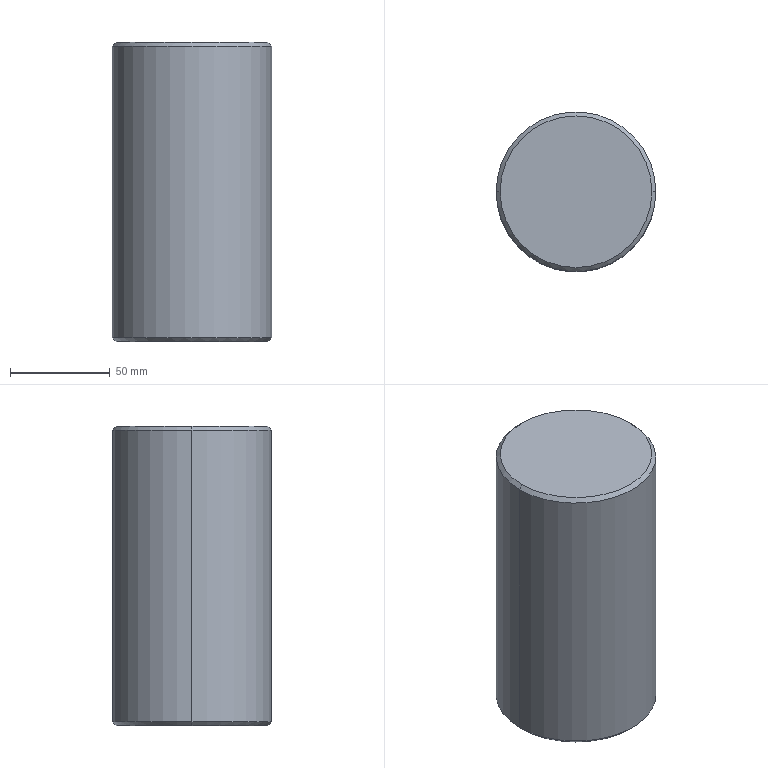Part | Creo | 1 solid | 15 faces | box 80 x 80 x 150 mm | volume 750871 mm3 | cylinder 6 | cone 6 | plane 3 | commonest cylinder face diameters 10.199 x2 10.2 x2 80 x2
STEP:
#1=CARTESIAN_POINT('',(-40.,-165.,-268.5));
#2=VERTEX_POINT('',#1);
#3=CARTESIAN_POINT('',(40.,-165.,-268.5));
#4=VERTEX_POINT('',#3);
#5=CARTESIAN_POINT('',(0.,-165.,-268.5));
#6=DIRECTION('',(0.,0.,-1.));
#7=DIRECTION('',(-1.,0.,0.));
#8=AXIS2_PLACEMENT_3D('',#5,#6,#7);
#9=CIRCLE('',#8,40.);
#10=EDGE_CURVE('',#2,#4,#9,.T.);
#11=ORIENTED_EDGE('',*,*,#10,.T.);
#12=CARTESIAN_POINT('',(40.,-165.,-122.5));
#13=VERTEX_POINT('',#12);
#14=CARTESIAN_POINT('',(40.,-165.,-122.5));
#15=DIRECTION('',(0.,0.,-1.));
#16=VECTOR('',#15,146.);
#17=LINE('',#14,#16);
#18=EDGE_CURVE('',#13,#4,#17,.T.);
#19=ORIENTED_EDGE('',*,*,#18,.F.);
#20=CARTESIAN_POINT('',(-40.,-165.,-122.5));
#21=VERTEX_POINT('',#20);
#22=CARTESIAN_POINT('',(0.,-165.,-122.5));
#23=DIRECTION('',(0.,0.,1.));
#24=DIRECTION('',(1.,0.,0.));
#25=AXIS2_PLACEMENT_3D('',#22,#23,#24);
#26=CIRCLE('',#25,40.);
#27=EDGE_CURVE('',#13,#21,#26,.T.);
#28=ORIENTED_EDGE('',*,*,#27,.T.);
#29=CARTESIAN_POINT('',(-40.,-165.,-122.5));
#30=DIRECTION('',(0.,0.,-1.));
#31=VECTOR('',#30,146.);
#32=LINE('',#29,#31);
#33=EDGE_CURVE('',#21,#2,#32,.T.);
#34=ORIENTED_EDGE('',*,*,#33,.T.);
#35=EDGE_LOOP('',(#11,#19,#28,#34));
#36=FACE_OUTER_BOUND('',#35,.F.);
#37=CARTESIAN_POINT('',(0.,-165.,-120.5));
#38=DIRECTION('',(0.,0.,-1.));
#39=DIRECTION('',(-1.,0.,0.));
#40=AXIS2_PLACEMENT_3D('',#37,#38,#39);
#41=CYLINDRICAL_SURFACE('',#40,40.);
#42=ADVANCED_FACE('',(#36),#41,.T.);
#43=CARTESIAN_POINT('',(-38.,-165.,-270.5));
#44=VERTEX_POINT('',#43);
#45=CARTESIAN_POINT('',(38.,-165.,-270.5));
#46=VERTEX_POINT('',#45);
#47=CARTESIAN_POINT('',(0.,-165.,-270.5));
#48=DIRECTION('',(0.,0.,-1.));
#49=DIRECTION('',(-1.,0.,0.));
#50=AXIS2_PLACEMENT_3D('',#47,#48,#49);
#51=CIRCLE('',#50,38.);
#52=EDGE_CURVE('',#44,#46,#51,.T.);
#53=ORIENTED_EDGE('',*,*,#52,.T.);
#54=CARTESIAN_POINT('',(38.,-165.,-270.5));
#55=DIRECTION('',(0.7071,0.,0.7071));
#56=VECTOR('',#55,2.828);
#57=LINE('',#54,#56);
#58=EDGE_CURVE('',#46,#4,#57,.T.);
#59=ORIENTED_EDGE('',*,*,#58,.T.);
#60=ORIENTED_EDGE('',*,*,#10,.F.);
#61=CARTESIAN_POINT('',(-38.,-165.,-270.5));
#62=DIRECTION('',(-0.7071,0.,0.7071));
#63=VECTOR('',#62,2.828);
#64=LINE('',#61,#63);
#65=EDGE_CURVE('',#44,#2,#64,.T.);
#66=ORIENTED_EDGE('',*,*,#65,.F.);
#67=EDGE_LOOP('',(#53,#59,#60,#66));
#68=FACE_OUTER_BOUND('',#67,.F.);
#69=CARTESIAN_POINT('',(0.,-165.,-269.5));
#70=DIRECTION('',(0.,0.,1.));
#71=DIRECTION('',(1.,0.,0.));
#72=AXIS2_PLACEMENT_3D('',#69,#70,#71);
#73=CONICAL_SURFACE('',#72,39.,45.);
#74=ADVANCED_FACE('',(#68),#73,.T.);
#75=CARTESIAN_POINT('',(0.,-165.,-270.5));
#76=DIRECTION('',(0.,0.,-1.));
#77=DIRECTION('',(1.,0.,0.));
#78=AXIS2_PLACEMENT_3D('',#75,#76,#77);
#79=CIRCLE('',#78,38.);
#80=EDGE_CURVE('',#46,#44,#79,.T.);
#81=ORIENTED_EDGE('',*,*,#80,.F.);
#82=ORIENTED_EDGE('',*,*,#52,.F.);
#83=EDGE_LOOP('',(#81,#82));
#84=FACE_OUTER_BOUND('',#83,.F.);
#85=CARTESIAN_POINT('',(5.1,-165.,-270.5));
#86=VERTEX_POINT('',#85);
#87=CARTESIAN_POINT('',(-5.1,-165.,-270.5));
#88=VERTEX_POINT('',#87);
#89=CARTESIAN_POINT('',(0.,-165.,-270.5));
#90=DIRECTION('',(0.,0.,1.));
#91=DIRECTION('',(1.,0.,0.));
#92=AXIS2_PLACEMENT_3D('',#89,#90,#91);
#93=CIRCLE('',#92,5.1);
#94=EDGE_CURVE('',#86,#88,#93,.T.);
#95=ORIENTED_EDGE('',*,*,#94,.F.);
#96=CARTESIAN_POINT('',(0.,-165.,-270.5));
#97=DIRECTION('',(0.,0.,1.));
#98=DIRECTION('',(-1.,0.,0.));
#99=AXIS2_PLACEMENT_3D('',#96,#97,#98);
#100=CIRCLE('',#99,5.1);
#101=EDGE_CURVE('',#88,#86,#100,.T.);
#102=ORIENTED_EDGE('',*,*,#101,.F.);
#103=EDGE_LOOP('',(#95,#102));
#104=FACE_BOUND('',#103,.F.);
#105=CARTESIAN_POINT('',(0.,-165.,-270.5));
#106=DIRECTION('',(0.,0.,1.));
#107=DIRECTION('',(1.,0.,0.));
#108=AXIS2_PLACEMENT_3D('',#105,#106,#107);
#109=PLANE('',#108);
#110=ADVANCED_FACE('',(#84,#104),#109,.F.);
#111=CARTESIAN_POINT('',(-5.1,-165.,-251.5));
#112=VERTEX_POINT('',#111);
#113=CARTESIAN_POINT('',(5.1,-165.,-251.5));
#114=VERTEX_POINT('',#113);
#115=CARTESIAN_POINT('',(0.,-165.,-251.5));
#116=DIRECTION('',(0.,0.,-1.));
#117=DIRECTION('',(-1.,0.,0.));
#118=AXIS2_PLACEMENT_3D('',#115,#116,#117);
#119=CIRCLE('',#118,5.099);
#120=EDGE_CURVE('',#112,#114,#119,.T.);
#121=ORIENTED_EDGE('',*,*,#120,.T.);
#122=CARTESIAN_POINT('',(5.1,-165.,-251.5));
#123=DIRECTION('',(0.00001316,0.,-1.));
#124=VECTOR('',#123,19.);
#125=LINE('',#122,#124);
#126=EDGE_CURVE('',#114,#86,#125,.T.);
#127=ORIENTED_EDGE('',*,*,#126,.T.);
#128=ORIENTED_EDGE('',*,*,#94,.T.);
#129=CARTESIAN_POINT('',(-5.1,-165.,-251.5));
#130=DIRECTION('',(-0.00001316,0.,-1.));
#131=VECTOR('',#130,19.);
#132=LINE('',#129,#131);
#133=EDGE_CURVE('',#112,#88,#132,.T.);
#134=ORIENTED_EDGE('',*,*,#133,.F.);
#135=EDGE_LOOP('',(#121,#127,#128,#134));
#136=FACE_OUTER_BOUND('',#135,.F.);
#137=CARTESIAN_POINT('',(0.,-165.,-251.5));
#138=DIRECTION('',(0.,0.,-1.));
#139=DIRECTION('',(-1.,0.,0.));
#140=AXIS2_PLACEMENT_3D('',#137,#138,#139);
#141=CYLINDRICAL_SURFACE('',#140,5.1);
#142=ADVANCED_FACE('',(#136),#141,.F.);
#143=CARTESIAN_POINT('',(-5.099,-165.,-245.5));
#144=VERTEX_POINT('',#143);
#145=CARTESIAN_POINT('',(5.099,-165.,-245.5));
#146=VERTEX_POINT('',#145);
#147=CARTESIAN_POINT('',(0.,-165.,-245.5));
#148=DIRECTION('',(0.,0.,-1.));
#149=DIRECTION('',(-1.,0.,0.));
#150=AXIS2_PLACEMENT_3D('',#147,#148,#149);
#151=CIRCLE('',#150,5.099);
#152=EDGE_CURVE('',#144,#146,#151,.T.);
#153=ORIENTED_EDGE('',*,*,#152,.T.);
#154=CARTESIAN_POINT('',(5.1,-165.,-251.5));
#155=DIRECTION('',(-0.00004167,0.,1.));
#156=VECTOR('',#155,6.);
#157=LINE('',#154,#156);
#158=EDGE_CURVE('',#114,#146,#157,.T.);
#159=ORIENTED_EDGE('',*,*,#158,.F.);
#160=ORIENTED_EDGE('',*,*,#120,.F.);
#161=CARTESIAN_POINT('',(-5.1,-165.,-251.5));
#162=DIRECTION('',(0.00004167,0.,1.));
#163=VECTOR('',#162,6.);
#164=LINE('',#161,#163);
#165=EDGE_CURVE('',#112,#144,#164,.T.);
#166=ORIENTED_EDGE('',*,*,#165,.T.);
#167=EDGE_LOOP('',(#153,#159,#160,#166));
#168=FACE_OUTER_BOUND('',#167,.F.);
#169=CARTESIAN_POINT('',(0.,-165.,-251.5));
#170=DIRECTION('',(0.,0.,1.));
#171=DIRECTION('',(1.,0.,0.));
#172=AXIS2_PLACEMENT_3D('',#169,#170,#171);
#173=CYLINDRICAL_SURFACE('',#172,5.099);
#174=ADVANCED_FACE('',(#168),#173,.F.);
#175=CARTESIAN_POINT('',(-0.2432,-165.,-242.696));
#176=VERTEX_POINT('',#175);
#177=CARTESIAN_POINT('',(0.2432,-165.,-242.696));
#178=VERTEX_POINT('',#177);
#179=CARTESIAN_POINT('',(0.,-165.,-242.696));
#180=DIRECTION('',(0.,0.,-1.));
#181=DIRECTION('',(-1.,0.,0.));
#182=AXIS2_PLACEMENT_3D('',#179,#180,#181);
#183=CIRCLE('',#182,0.2432);
#184=EDGE_CURVE('',#176,#178,#183,.T.);
#185=ORIENTED_EDGE('',*,*,#184,.T.);
#186=CARTESIAN_POINT('',(0.2432,-165.,-242.696));
#187=DIRECTION('',(0.866,0.,-0.5));
#188=VECTOR('',#187,5.608);
#189=LINE('',#186,#188);
#190=EDGE_CURVE('',#178,#146,#189,.T.);
#191=ORIENTED_EDGE('',*,*,#190,.T.);
#192=ORIENTED_EDGE('',*,*,#152,.F.);
#193=CARTESIAN_POINT('',(-0.2432,-165.,-242.696));
#194=DIRECTION('',(-0.866,0.,-0.5));
#195=VECTOR('',#194,5.608);
#196=LINE('',#193,#195);
#197=EDGE_CURVE('',#176,#144,#196,.T.);
#198=ORIENTED_EDGE('',*,*,#197,.F.);
#199=EDGE_LOOP('',(#185,#191,#192,#198));
#200=FACE_OUTER_BOUND('',#199,.F.);
#201=CARTESIAN_POINT('',(0.,-165.,-244.098));
#202=DIRECTION('',(0.,0.,-1.));
#203=DIRECTION('',(-1.,0.,0.));
#204=AXIS2_PLACEMENT_3D('',#201,#202,#203);
#205=CONICAL_SURFACE('',#204,2.671,60.);
#206=ADVANCED_FACE('',(#200),#205,.F.);
#207=CARTESIAN_POINT('',(0.,-165.,-242.696));
#208=DIRECTION('',(0.,0.,-1.));
#209=DIRECTION('',(1.,0.,0.));
#210=AXIS2_PLACEMENT_3D('',#207,#208,#209);
#211=CIRCLE('',#210,0.2432);
#212=EDGE_CURVE('',#178,#176,#211,.T.);
#213=ORIENTED_EDGE('',*,*,#212,.F.);
#214=ORIENTED_EDGE('',*,*,#184,.F.);
#215=EDGE_LOOP('',(#213,#214));
#216=FACE_OUTER_BOUND('',#215,.F.);
#217=CARTESIAN_POINT('',(0.,-165.,-242.696));
#218=DIRECTION('',(0.,0.,1.));
#219=DIRECTION('',(1.,0.,0.));
#220=AXIS2_PLACEMENT_3D('',#217,#218,#219);
#221=PLANE('',#220);
#222=ADVANCED_FACE('',(#216),#221,.F.);
#223=ORIENTED_EDGE('',*,*,#212,.T.);
#224=ORIENTED_EDGE('',*,*,#197,.T.);
#225=CARTESIAN_POINT('',(0.,-165.,-245.5));
#226=DIRECTION('',(0.,0.,-1.));
#227=DIRECTION('',(1.,0.,0.));
#228=AXIS2_PLACEMENT_3D('',#225,#226,#227);
#229=CIRCLE('',#228,5.099);
#230=EDGE_CURVE('',#146,#144,#229,.T.);
#231=ORIENTED_EDGE('',*,*,#230,.F.);
#232=ORIENTED_EDGE('',*,*,#190,.F.);
#233=EDGE_LOOP('',(#223,#224,#231,#232));
#234=FACE_OUTER_BOUND('',#233,.F.);
#235=CARTESIAN_POINT('',(0.,-165.,-244.098));
#236=DIRECTION('',(0.,0.,-1.));
#237=DIRECTION('',(-1.,0.,0.));
#238=AXIS2_PLACEMENT_3D('',#235,#236,#237);
#239=CONICAL_SURFACE('',#238,2.671,60.);
#240=ADVANCED_FACE('',(#234),#239,.F.);
#241=ORIENTED_EDGE('',*,*,#230,.T.);
#242=ORIENTED_EDGE('',*,*,#165,.F.);
#243=CARTESIAN_POINT('',(0.,-165.,-251.5));
#244=DIRECTION('',(0.,0.,-1.));
#245=DIRECTION('',(1.,0.,0.));
#246=AXIS2_PLACEMENT_3D('',#243,#244,#245);
#247=CIRCLE('',#246,5.099);
#248=EDGE_CURVE('',#114,#112,#247,.T.);
#249=ORIENTED_EDGE('',*,*,#248,.F.);
#250=ORIENTED_EDGE('',*,*,#158,.T.);
#251=EDGE_LOOP('',(#241,#242,#249,#250));
#252=FACE_OUTER_BOUND('',#251,.F.);
#253=CARTESIAN_POINT('',(0.,-165.,-251.5));
#254=DIRECTION('',(0.,0.,1.));
#255=DIRECTION('',(1.,0.,0.));
#256=AXIS2_PLACEMENT_3D('',#253,#254,#255);
#257=CYLINDRICAL_SURFACE('',#256,5.099);
#258=ADVANCED_FACE('',(#252),#257,.F.);
#259=ORIENTED_EDGE('',*,*,#248,.T.);
#260=ORIENTED_EDGE('',*,*,#133,.T.);
#261=ORIENTED_EDGE('',*,*,#101,.T.);
#262=ORIENTED_EDGE('',*,*,#126,.F.);
#263=EDGE_LOOP('',(#259,#260,#261,#262));
#264=FACE_OUTER_BOUND('',#263,.F.);
#265=CARTESIAN_POINT('',(0.,-165.,-251.5));
#266=DIRECTION('',(0.,0.,-1.));
#267=DIRECTION('',(-1.,0.,0.));
#268=AXIS2_PLACEMENT_3D('',#265,#266,#267);
#269=CYLINDRICAL_SURFACE('',#268,5.1);
#270=ADVANCED_FACE('',(#264),#269,.F.);
#271=ORIENTED_EDGE('',*,*,#80,.T.);
#272=ORIENTED_EDGE('',*,*,#65,.T.);
#273=CARTESIAN_POINT('',(0.,-165.,-268.5));
#274=DIRECTION('',(0.,0.,-1.));
#275=DIRECTION('',(1.,0.,0.));
#276=AXIS2_PLACEMENT_3D('',#273,#274,#275);
#277=CIRCLE('',#276,40.);
#278=EDGE_CURVE('',#4,#2,#277,.T.);
#279=ORIENTED_EDGE('',*,*,#278,.F.);
#280=ORIENTED_EDGE('',*,*,#58,.F.);
#281=EDGE_LOOP('',(#271,#272,#279,#280));
#282=FACE_OUTER_BOUND('',#281,.F.);
#283=CARTESIAN_POINT('',(0.,-165.,-269.5));
#284=DIRECTION('',(0.,0.,1.));
#285=DIRECTION('',(1.,0.,0.));
#286=AXIS2_PLACEMENT_3D('',#283,#284,#285);
#287=CONICAL_SURFACE('',#286,39.,45.);
#288=ADVANCED_FACE('',(#282),#287,.T.);
#289=ORIENTED_EDGE('',*,*,#278,.T.);
#290=ORIENTED_EDGE('',*,*,#33,.F.);
#291=CARTESIAN_POINT('',(0.,-165.,-122.5));
#292=DIRECTION('',(0.,0.,1.));
#293=DIRECTION('',(-1.,0.,0.));
#294=AXIS2_PLACEMENT_3D('',#291,#292,#293);
#295=CIRCLE('',#294,40.);
#296=EDGE_CURVE('',#21,#13,#295,.T.);
#297=ORIENTED_EDGE('',*,*,#296,.T.);
#298=ORIENTED_EDGE('',*,*,#18,.T.);
#299=EDGE_LOOP('',(#289,#290,#297,#298));
#300=FACE_OUTER_BOUND('',#299,.F.);
#301=CARTESIAN_POINT('',(0.,-165.,-120.5));
#302=DIRECTION('',(0.,0.,-1.));
#303=DIRECTION('',(-1.,0.,0.));
#304=AXIS2_PLACEMENT_3D('',#301,#302,#303);
#305=CYLINDRICAL_SURFACE('',#304,40.);
#306=ADVANCED_FACE('',(#300),#305,.T.);
#307=ORIENTED_EDGE('',*,*,#296,.F.);
#308=CARTESIAN_POINT('',(-38.,-165.,-120.5));
#309=VERTEX_POINT('',#308);
#310=CARTESIAN_POINT('',(-38.,-165.,-120.5));
#311=DIRECTION('',(-0.7071,0.,-0.7071));
#312=VECTOR('',#311,2.828);
#313=LINE('',#310,#312);
#314=EDGE_CURVE('',#309,#21,#313,.T.);
#315=ORIENTED_EDGE('',*,*,#314,.F.);
#316=CARTESIAN_POINT('',(38.,-165.,-120.5));
#317=VERTEX_POINT('',#316);
#318=CARTESIAN_POINT('',(0.,-165.,-120.5));
#319=DIRECTION('',(0.,0.,1.));
#320=DIRECTION('',(-1.,0.,0.));
#321=AXIS2_PLACEMENT_3D('',#318,#319,#320);
#322=CIRCLE('',#321,38.);
#323=EDGE_CURVE('',#309,#317,#322,.T.);
#324=ORIENTED_EDGE('',*,*,#323,.T.);
#325=CARTESIAN_POINT('',(38.,-165.,-120.5));
#326=DIRECTION('',(0.7071,0.,-0.7071));
#327=VECTOR('',#326,2.828);
#328=LINE('',#325,#327);
#329=EDGE_CURVE('',#317,#13,#328,.T.);
#330=ORIENTED_EDGE('',*,*,#329,.T.);
#331=EDGE_LOOP('',(#307,#315,#324,#330));
#332=FACE_OUTER_BOUND('',#331,.F.);
#333=CARTESIAN_POINT('',(0.,-165.,-121.5));
#334=DIRECTION('',(0.,0.,-1.));
#335=DIRECTION('',(-1.,0.,0.));
#336=AXIS2_PLACEMENT_3D('',#333,#334,#335);
#337=CONICAL_SURFACE('',#336,39.,45.);
#338=ADVANCED_FACE('',(#332),#337,.T.);
#339=ORIENTED_EDGE('',*,*,#27,.F.);
#340=ORIENTED_EDGE('',*,*,#329,.F.);
#341=CARTESIAN_POINT('',(0.,-165.,-120.5));
#342=DIRECTION('',(0.,0.,1.));
#343=DIRECTION('',(1.,0.,0.));
#344=AXIS2_PLACEMENT_3D('',#341,#342,#343);
#345=CIRCLE('',#344,38.);
#346=EDGE_CURVE('',#317,#309,#345,.T.);
#347=ORIENTED_EDGE('',*,*,#346,.T.);
#348=ORIENTED_EDGE('',*,*,#314,.T.);
#349=EDGE_LOOP('',(#339,#340,#347,#348));
#350=FACE_OUTER_BOUND('',#349,.F.);
#351=CARTESIAN_POINT('',(0.,-165.,-121.5));
#352=DIRECTION('',(0.,0.,-1.));
#353=DIRECTION('',(-1.,0.,0.));
#354=AXIS2_PLACEMENT_3D('',#351,#352,#353);
#355=CONICAL_SURFACE('',#354,39.,45.);
#356=ADVANCED_FACE('',(#350),#355,.T.);
#357=ORIENTED_EDGE('',*,*,#346,.F.);
#358=ORIENTED_EDGE('',*,*,#323,.F.);
#359=EDGE_LOOP('',(#357,#358));
#360=FACE_OUTER_BOUND('',#359,.F.);
#361=CARTESIAN_POINT('',(0.,-165.,-120.5));
#362=DIRECTION('',(0.,0.,1.));
#363=DIRECTION('',(1.,0.,0.));
#364=AXIS2_PLACEMENT_3D('',#361,#362,#363);
#365=PLANE('',#364);
#366=ADVANCED_FACE('',(#360),#365,.T.);
#367=CLOSED_SHELL('',(#42,#74,#110,#142,#174,#206,#222,#240,#258,#270,#288,#306,#338,#356,#366));
#368=MANIFOLD_SOLID_BREP('',#367);
#369=(LENGTH_UNIT()NAMED_UNIT(*)SI_UNIT(.MILLI.,.METRE.));
#370=UNCERTAINTY_MEASURE_WITH_UNIT(LENGTH_MEASURE(0.01879),#369,'','');
#371=(NAMED_UNIT(*)PLANE_ANGLE_UNIT()SI_UNIT($,.RADIAN.));
#372=PLANE_ANGLE_MEASURE_WITH_UNIT(PLANE_ANGLE_MEASURE(0.01745),#371);
#373=(CONVERSION_BASED_UNIT('DEGREE',#372)NAMED_UNIT(*)PLANE_ANGLE_UNIT());
#374=(NAMED_UNIT(*)SI_UNIT($,.STERADIAN.)SOLID_ANGLE_UNIT());
#375=(GEOMETRIC_REPRESENTATION_CONTEXT(3)GLOBAL_UNCERTAINTY_ASSIGNED_CONTEXT((#370))GLOBAL_UNIT_ASSIGNED_CONTEXT((#369,#373,#374))REPRESENTATION_CONTEXT('',''));
#376=ADVANCED_BREP_SHAPE_REPRESENTATION('',(#368),#375);